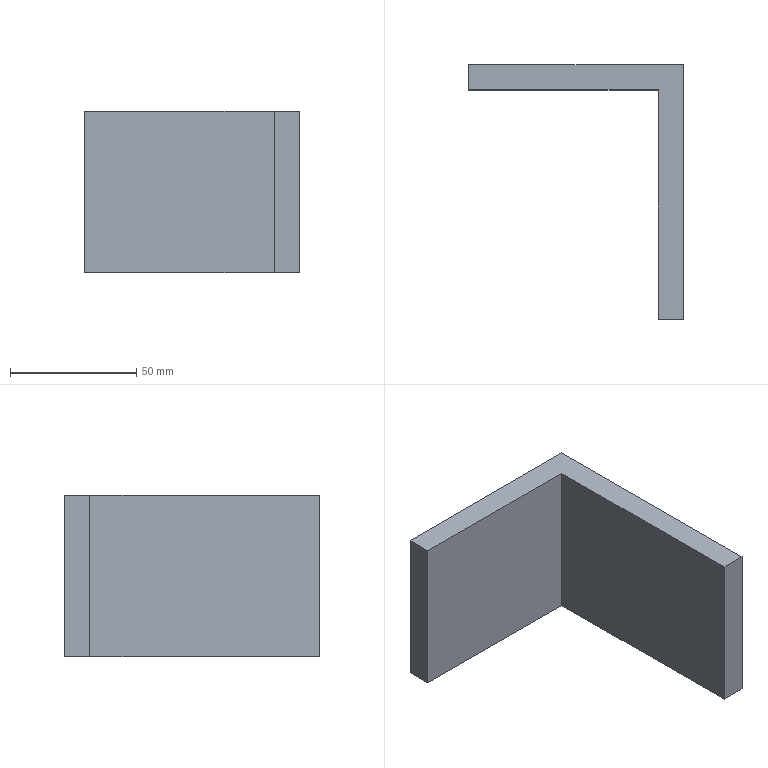Part | STEP file | Cylinder support plate | 1 solid | 8 faces | box 85 x 100.75 x 64 mm | volume 112480 mm3 | plane 8
STEP:
#1=CARTESIAN_POINT('',(0.,0.,0.));
#2=DIRECTION('',(0.,0.,1.));
#3=DIRECTION('',(1.,0.,0.));
#4=AXIS2_PLACEMENT_3D('',#1,#2,#3);
#5=CARTESIAN_POINT('',(85.,10.,64.));
#6=VERTEX_POINT('',#5);
#7=CARTESIAN_POINT('',(85.,10.,0.));
#8=VERTEX_POINT('',#7);
#9=CARTESIAN_POINT('',(85.,10.,64.));
#10=DIRECTION('',(0.,0.,-1.));
#11=VECTOR('',#10,1.);
#12=LINE('',#9,#11);
#13=CARTESIAN_POINT('',(85.,-90.75,64.));
#14=DIRECTION('',(-1.,0.,0.));
#15=DIRECTION('',(0.,0.,1.));
#16=AXIS2_PLACEMENT_3D('',#13,#14,#15);
#17=PLANE('',#16);
#18=CARTESIAN_POINT('',(0.,100.75));
#19=DIRECTION('',(-1.,0.));
#20=VECTOR('',#19,1.);
#21=LINE('',#18,#20);
#22=(GEOMETRIC_REPRESENTATION_CONTEXT(2)PARAMETRIC_REPRESENTATION_CONTEXT()REPRESENTATION_CONTEXT('',''));
#23=DEFINITIONAL_REPRESENTATION('',(#21),#22);
#24=PCURVE('',#17,#23);
#25=CARTESIAN_POINT('',(85.,10.,64.));
#26=DIRECTION('',(0.,-1.,0.));
#27=DIRECTION('',(1.,0.,0.));
#28=AXIS2_PLACEMENT_3D('',#25,#26,#27);
#29=PLANE('',#28);
#30=CARTESIAN_POINT('',(0.,0.));
#31=DIRECTION('',(0.,-1.));
#32=VECTOR('',#31,1.);
#33=LINE('',#30,#32);
#34=(GEOMETRIC_REPRESENTATION_CONTEXT(2)PARAMETRIC_REPRESENTATION_CONTEXT()REPRESENTATION_CONTEXT('',''));
#35=DEFINITIONAL_REPRESENTATION('',(#33),#34);
#36=PCURVE('',#29,#35);
#37=SURFACE_CURVE('',#12,(#24,#36),.PCURVE_S1.);
#38=EDGE_CURVE('',#6,#8,#37,.T.);
#39=ORIENTED_EDGE('',*,*,#38,.F.);
#40=CARTESIAN_POINT('',(85.,-90.75,64.));
#41=VERTEX_POINT('',#40);
#42=CARTESIAN_POINT('',(85.,-90.75,64.));
#43=DIRECTION('',(0.,1.,0.));
#44=VECTOR('',#43,1.);
#45=LINE('',#42,#44);
#46=CARTESIAN_POINT('',(0.,0.));
#47=DIRECTION('',(0.,1.));
#48=VECTOR('',#47,1.);
#49=LINE('',#46,#48);
#50=(GEOMETRIC_REPRESENTATION_CONTEXT(2)PARAMETRIC_REPRESENTATION_CONTEXT()REPRESENTATION_CONTEXT('',''));
#51=DEFINITIONAL_REPRESENTATION('',(#49),#50);
#52=PCURVE('',#17,#51);
#53=CARTESIAN_POINT('',(0.,0.,64.));
#54=DIRECTION('',(0.,0.,1.));
#55=DIRECTION('',(1.,0.,0.));
#56=AXIS2_PLACEMENT_3D('',#53,#54,#55);
#57=PLANE('',#56);
#58=CARTESIAN_POINT('',(85.,-90.75));
#59=DIRECTION('',(0.,1.));
#60=VECTOR('',#59,1.);
#61=LINE('',#58,#60);
#62=(GEOMETRIC_REPRESENTATION_CONTEXT(2)PARAMETRIC_REPRESENTATION_CONTEXT()REPRESENTATION_CONTEXT('',''));
#63=DEFINITIONAL_REPRESENTATION('',(#61),#62);
#64=PCURVE('',#57,#63);
#65=SURFACE_CURVE('',#45,(#52,#64),.PCURVE_S1.);
#66=EDGE_CURVE('',#41,#6,#65,.T.);
#67=ORIENTED_EDGE('',*,*,#66,.F.);
#68=CARTESIAN_POINT('',(85.,-90.75,0.));
#69=VERTEX_POINT('',#68);
#70=CARTESIAN_POINT('',(85.,-90.75,64.));
#71=DIRECTION('',(0.,0.,1.));
#72=VECTOR('',#71,1.);
#73=LINE('',#70,#72);
#74=CARTESIAN_POINT('',(0.,0.));
#75=DIRECTION('',(1.,0.));
#76=VECTOR('',#75,1.);
#77=LINE('',#74,#76);
#78=(GEOMETRIC_REPRESENTATION_CONTEXT(2)PARAMETRIC_REPRESENTATION_CONTEXT()REPRESENTATION_CONTEXT('',''));
#79=DEFINITIONAL_REPRESENTATION('',(#77),#78);
#80=PCURVE('',#17,#79);
#81=CARTESIAN_POINT('',(75.,-90.75,64.));
#82=DIRECTION('',(0.,1.,0.));
#83=DIRECTION('',(0.,0.,1.));
#84=AXIS2_PLACEMENT_3D('',#81,#82,#83);
#85=PLANE('',#84);
#86=CARTESIAN_POINT('',(0.,10.));
#87=DIRECTION('',(1.,0.));
#88=VECTOR('',#87,1.);
#89=LINE('',#86,#88);
#90=(GEOMETRIC_REPRESENTATION_CONTEXT(2)PARAMETRIC_REPRESENTATION_CONTEXT()REPRESENTATION_CONTEXT('',''));
#91=DEFINITIONAL_REPRESENTATION('',(#89),#90);
#92=PCURVE('',#85,#91);
#93=SURFACE_CURVE('',#73,(#80,#92),.PCURVE_S1.);
#94=EDGE_CURVE('',#69,#41,#93,.T.);
#95=ORIENTED_EDGE('',*,*,#94,.F.);
#96=CARTESIAN_POINT('',(85.,-90.75,0.));
#97=DIRECTION('',(0.,-1.,0.));
#98=VECTOR('',#97,1.);
#99=LINE('',#96,#98);
#100=CARTESIAN_POINT('',(-64.,0.));
#101=DIRECTION('',(0.,-1.));
#102=VECTOR('',#101,1.);
#103=LINE('',#100,#102);
#104=(GEOMETRIC_REPRESENTATION_CONTEXT(2)PARAMETRIC_REPRESENTATION_CONTEXT()REPRESENTATION_CONTEXT('',''));
#105=DEFINITIONAL_REPRESENTATION('',(#103),#104);
#106=PCURVE('',#17,#105);
#107=CARTESIAN_POINT('',(0.,0.,0.));
#108=DIRECTION('',(0.,0.,1.));
#109=DIRECTION('',(1.,0.,0.));
#110=AXIS2_PLACEMENT_3D('',#107,#108,#109);
#111=PLANE('',#110);
#112=CARTESIAN_POINT('',(85.,-90.75));
#113=DIRECTION('',(0.,-1.));
#114=VECTOR('',#113,1.);
#115=LINE('',#112,#114);
#116=(GEOMETRIC_REPRESENTATION_CONTEXT(2)PARAMETRIC_REPRESENTATION_CONTEXT()REPRESENTATION_CONTEXT('',''));
#117=DEFINITIONAL_REPRESENTATION('',(#115),#116);
#118=PCURVE('',#111,#117);
#119=SURFACE_CURVE('',#99,(#106,#118),.PCURVE_S1.);
#120=EDGE_CURVE('',#8,#69,#119,.T.);
#121=ORIENTED_EDGE('',*,*,#120,.F.);
#122=EDGE_LOOP('',(#39,#67,#95,#121));
#123=FACE_BOUND('',#122,.T.);
#124=ADVANCED_FACE('',(#123),#17,.F.);
#125=CARTESIAN_POINT('',(0.,10.,0.));
#126=VERTEX_POINT('',#125);
#127=CARTESIAN_POINT('',(0.,10.,0.));
#128=DIRECTION('',(-1.,0.,0.));
#129=VECTOR('',#128,1.);
#130=LINE('',#127,#129);
#131=CARTESIAN_POINT('',(0.,10.));
#132=DIRECTION('',(-1.,0.));
#133=VECTOR('',#132,1.);
#134=LINE('',#131,#133);
#135=(GEOMETRIC_REPRESENTATION_CONTEXT(2)PARAMETRIC_REPRESENTATION_CONTEXT()REPRESENTATION_CONTEXT('',''));
#136=DEFINITIONAL_REPRESENTATION('',(#134),#135);
#137=PCURVE('',#111,#136);
#138=CARTESIAN_POINT('',(-85.,-64.));
#139=DIRECTION('',(-1.,0.));
#140=VECTOR('',#139,1.);
#141=LINE('',#138,#140);
#142=(GEOMETRIC_REPRESENTATION_CONTEXT(2)PARAMETRIC_REPRESENTATION_CONTEXT()REPRESENTATION_CONTEXT('',''));
#143=DEFINITIONAL_REPRESENTATION('',(#141),#142);
#144=PCURVE('',#29,#143);
#145=SURFACE_CURVE('',#130,(#137,#144),.PCURVE_S1.);
#146=EDGE_CURVE('',#8,#126,#145,.T.);
#147=ORIENTED_EDGE('',*,*,#146,.F.);
#148=ORIENTED_EDGE('',*,*,#120,.T.);
#149=CARTESIAN_POINT('',(75.,-90.75,0.));
#150=VERTEX_POINT('',#149);
#151=CARTESIAN_POINT('',(0.,-90.75,0.));
#152=DIRECTION('',(1.,0.,0.));
#153=VECTOR('',#152,1.);
#154=LINE('',#151,#153);
#155=CARTESIAN_POINT('',(0.,-90.75));
#156=DIRECTION('',(1.,0.));
#157=VECTOR('',#156,1.);
#158=LINE('',#155,#157);
#159=(GEOMETRIC_REPRESENTATION_CONTEXT(2)PARAMETRIC_REPRESENTATION_CONTEXT()REPRESENTATION_CONTEXT('',''));
#160=DEFINITIONAL_REPRESENTATION('',(#158),#159);
#161=PCURVE('',#111,#160);
#162=CARTESIAN_POINT('',(-64.,-75.));
#163=DIRECTION('',(0.,1.));
#164=VECTOR('',#163,1.);
#165=LINE('',#162,#164);
#166=(GEOMETRIC_REPRESENTATION_CONTEXT(2)PARAMETRIC_REPRESENTATION_CONTEXT()REPRESENTATION_CONTEXT('',''));
#167=DEFINITIONAL_REPRESENTATION('',(#165),#166);
#168=PCURVE('',#85,#167);
#169=SURFACE_CURVE('',#154,(#161,#168),.PCURVE_S1.);
#170=EDGE_CURVE('',#150,#69,#169,.T.);
#171=ORIENTED_EDGE('',*,*,#170,.F.);
#172=CARTESIAN_POINT('',(75.,0.,0.));
#173=VERTEX_POINT('',#172);
#174=CARTESIAN_POINT('',(75.,0.,0.));
#175=DIRECTION('',(0.,-1.,0.));
#176=VECTOR('',#175,1.);
#177=LINE('',#174,#176);
#178=CARTESIAN_POINT('',(75.,0.));
#179=DIRECTION('',(0.,-1.));
#180=VECTOR('',#179,1.);
#181=LINE('',#178,#180);
#182=(GEOMETRIC_REPRESENTATION_CONTEXT(2)PARAMETRIC_REPRESENTATION_CONTEXT()REPRESENTATION_CONTEXT('',''));
#183=DEFINITIONAL_REPRESENTATION('',(#181),#182);
#184=PCURVE('',#111,#183);
#185=CARTESIAN_POINT('',(75.,0.,64.));
#186=DIRECTION('',(1.,0.,0.));
#187=DIRECTION('',(0.,1.,0.));
#188=AXIS2_PLACEMENT_3D('',#185,#186,#187);
#189=PLANE('',#188);
#190=CARTESIAN_POINT('',(0.,-64.));
#191=DIRECTION('',(-1.,0.));
#192=VECTOR('',#191,1.);
#193=LINE('',#190,#192);
#194=(GEOMETRIC_REPRESENTATION_CONTEXT(2)PARAMETRIC_REPRESENTATION_CONTEXT()REPRESENTATION_CONTEXT('',''));
#195=DEFINITIONAL_REPRESENTATION('',(#193),#194);
#196=PCURVE('',#189,#195);
#197=SURFACE_CURVE('',#177,(#184,#196),.PCURVE_S1.);
#198=EDGE_CURVE('',#173,#150,#197,.T.);
#199=ORIENTED_EDGE('',*,*,#198,.F.);
#200=CARTESIAN_POINT('',(0.,0.,0.));
#201=VERTEX_POINT('',#200);
#202=CARTESIAN_POINT('',(0.,0.,0.));
#203=DIRECTION('',(1.,0.,0.));
#204=VECTOR('',#203,1.);
#205=LINE('',#202,#204);
#206=CARTESIAN_POINT('',(0.,0.));
#207=DIRECTION('',(1.,0.));
#208=VECTOR('',#207,1.);
#209=LINE('',#206,#208);
#210=(GEOMETRIC_REPRESENTATION_CONTEXT(2)PARAMETRIC_REPRESENTATION_CONTEXT()REPRESENTATION_CONTEXT('',''));
#211=DEFINITIONAL_REPRESENTATION('',(#209),#210);
#212=PCURVE('',#111,#211);
#213=CARTESIAN_POINT('',(0.,0.,64.));
#214=DIRECTION('',(0.,1.,0.));
#215=DIRECTION('',(0.,0.,1.));
#216=AXIS2_PLACEMENT_3D('',#213,#214,#215);
#217=PLANE('',#216);
#218=CARTESIAN_POINT('',(-64.,0.));
#219=DIRECTION('',(0.,1.));
#220=VECTOR('',#219,1.);
#221=LINE('',#218,#220);
#222=(GEOMETRIC_REPRESENTATION_CONTEXT(2)PARAMETRIC_REPRESENTATION_CONTEXT()REPRESENTATION_CONTEXT('',''));
#223=DEFINITIONAL_REPRESENTATION('',(#221),#222);
#224=PCURVE('',#217,#223);
#225=SURFACE_CURVE('',#205,(#212,#224),.PCURVE_S1.);
#226=EDGE_CURVE('',#201,#173,#225,.T.);
#227=ORIENTED_EDGE('',*,*,#226,.F.);
#228=CARTESIAN_POINT('',(0.,0.,0.));
#229=DIRECTION('',(0.,-1.,0.));
#230=VECTOR('',#229,1.);
#231=LINE('',#228,#230);
#232=CARTESIAN_POINT('',(0.,0.));
#233=DIRECTION('',(0.,-1.));
#234=VECTOR('',#233,1.);
#235=LINE('',#232,#234);
#236=(GEOMETRIC_REPRESENTATION_CONTEXT(2)PARAMETRIC_REPRESENTATION_CONTEXT()REPRESENTATION_CONTEXT('',''));
#237=DEFINITIONAL_REPRESENTATION('',(#235),#236);
#238=PCURVE('',#111,#237);
#239=CARTESIAN_POINT('',(0.,10.,64.));
#240=DIRECTION('',(1.,0.,0.));
#241=DIRECTION('',(0.,1.,0.));
#242=AXIS2_PLACEMENT_3D('',#239,#240,#241);
#243=PLANE('',#242);
#244=CARTESIAN_POINT('',(-10.,-64.));
#245=DIRECTION('',(-1.,0.));
#246=VECTOR('',#245,1.);
#247=LINE('',#244,#246);
#248=(GEOMETRIC_REPRESENTATION_CONTEXT(2)PARAMETRIC_REPRESENTATION_CONTEXT()REPRESENTATION_CONTEXT('',''));
#249=DEFINITIONAL_REPRESENTATION('',(#247),#248);
#250=PCURVE('',#243,#249);
#251=SURFACE_CURVE('',#231,(#238,#250),.PCURVE_S1.);
#252=EDGE_CURVE('',#126,#201,#251,.T.);
#253=ORIENTED_EDGE('',*,*,#252,.F.);
#254=EDGE_LOOP('',(#147,#148,#171,#199,#227,#253));
#255=FACE_BOUND('',#254,.T.);
#256=ADVANCED_FACE('',(#255),#111,.F.);
#257=CARTESIAN_POINT('',(0.,10.,64.));
#258=VERTEX_POINT('',#257);
#259=CARTESIAN_POINT('',(0.,10.,64.));
#260=DIRECTION('',(0.,0.,-1.));
#261=VECTOR('',#260,1.);
#262=LINE('',#259,#261);
#263=CARTESIAN_POINT('',(-85.,0.));
#264=DIRECTION('',(0.,-1.));
#265=VECTOR('',#264,1.);
#266=LINE('',#263,#265);
#267=(GEOMETRIC_REPRESENTATION_CONTEXT(2)PARAMETRIC_REPRESENTATION_CONTEXT()REPRESENTATION_CONTEXT('',''));
#268=DEFINITIONAL_REPRESENTATION('',(#266),#267);
#269=PCURVE('',#29,#268);
#270=CARTESIAN_POINT('',(0.,0.));
#271=DIRECTION('',(0.,-1.));
#272=VECTOR('',#271,1.);
#273=LINE('',#270,#272);
#274=(GEOMETRIC_REPRESENTATION_CONTEXT(2)PARAMETRIC_REPRESENTATION_CONTEXT()REPRESENTATION_CONTEXT('',''));
#275=DEFINITIONAL_REPRESENTATION('',(#273),#274);
#276=PCURVE('',#243,#275);
#277=SURFACE_CURVE('',#262,(#269,#276),.PCURVE_S1.);
#278=EDGE_CURVE('',#258,#126,#277,.T.);
#279=ORIENTED_EDGE('',*,*,#278,.F.);
#280=CARTESIAN_POINT('',(85.,10.,64.));
#281=DIRECTION('',(-1.,0.,0.));
#282=VECTOR('',#281,1.);
#283=LINE('',#280,#282);
#284=CARTESIAN_POINT('',(0.,0.));
#285=DIRECTION('',(-1.,0.));
#286=VECTOR('',#285,1.);
#287=LINE('',#284,#286);
#288=(GEOMETRIC_REPRESENTATION_CONTEXT(2)PARAMETRIC_REPRESENTATION_CONTEXT()REPRESENTATION_CONTEXT('',''));
#289=DEFINITIONAL_REPRESENTATION('',(#287),#288);
#290=PCURVE('',#29,#289);
#291=CARTESIAN_POINT('',(85.,10.));
#292=DIRECTION('',(-1.,0.));
#293=VECTOR('',#292,1.);
#294=LINE('',#291,#293);
#295=(GEOMETRIC_REPRESENTATION_CONTEXT(2)PARAMETRIC_REPRESENTATION_CONTEXT()REPRESENTATION_CONTEXT('',''));
#296=DEFINITIONAL_REPRESENTATION('',(#294),#295);
#297=PCURVE('',#57,#296);
#298=SURFACE_CURVE('',#283,(#290,#297),.PCURVE_S1.);
#299=EDGE_CURVE('',#6,#258,#298,.T.);
#300=ORIENTED_EDGE('',*,*,#299,.F.);
#301=ORIENTED_EDGE('',*,*,#38,.T.);
#302=ORIENTED_EDGE('',*,*,#146,.T.);
#303=EDGE_LOOP('',(#279,#300,#301,#302));
#304=FACE_BOUND('',#303,.T.);
#305=ADVANCED_FACE('',(#304),#29,.F.);
#306=ORIENTED_EDGE('',*,*,#66,.T.);
#307=ORIENTED_EDGE('',*,*,#299,.T.);
#308=CARTESIAN_POINT('',(0.,0.,64.));
#309=VERTEX_POINT('',#308);
#310=CARTESIAN_POINT('',(0.,0.,64.));
#311=DIRECTION('',(0.,-1.,0.));
#312=VECTOR('',#311,1.);
#313=LINE('',#310,#312);
#314=CARTESIAN_POINT('',(0.,0.));
#315=DIRECTION('',(0.,-1.));
#316=VECTOR('',#315,1.);
#317=LINE('',#314,#316);
#318=(GEOMETRIC_REPRESENTATION_CONTEXT(2)PARAMETRIC_REPRESENTATION_CONTEXT()REPRESENTATION_CONTEXT('',''));
#319=DEFINITIONAL_REPRESENTATION('',(#317),#318);
#320=PCURVE('',#57,#319);
#321=CARTESIAN_POINT('',(-10.,0.));
#322=DIRECTION('',(-1.,0.));
#323=VECTOR('',#322,1.);
#324=LINE('',#321,#323);
#325=(GEOMETRIC_REPRESENTATION_CONTEXT(2)PARAMETRIC_REPRESENTATION_CONTEXT()REPRESENTATION_CONTEXT('',''));
#326=DEFINITIONAL_REPRESENTATION('',(#324),#325);
#327=PCURVE('',#243,#326);
#328=SURFACE_CURVE('',#313,(#320,#327),.PCURVE_S1.);
#329=EDGE_CURVE('',#258,#309,#328,.T.);
#330=ORIENTED_EDGE('',*,*,#329,.T.);
#331=CARTESIAN_POINT('',(75.,0.,64.));
#332=VERTEX_POINT('',#331);
#333=CARTESIAN_POINT('',(0.,0.,64.));
#334=DIRECTION('',(1.,0.,0.));
#335=VECTOR('',#334,1.);
#336=LINE('',#333,#335);
#337=CARTESIAN_POINT('',(0.,0.));
#338=DIRECTION('',(1.,0.));
#339=VECTOR('',#338,1.);
#340=LINE('',#337,#339);
#341=(GEOMETRIC_REPRESENTATION_CONTEXT(2)PARAMETRIC_REPRESENTATION_CONTEXT()REPRESENTATION_CONTEXT('',''));
#342=DEFINITIONAL_REPRESENTATION('',(#340),#341);
#343=PCURVE('',#57,#342);
#344=CARTESIAN_POINT('',(0.,0.));
#345=DIRECTION('',(0.,1.));
#346=VECTOR('',#345,1.);
#347=LINE('',#344,#346);
#348=(GEOMETRIC_REPRESENTATION_CONTEXT(2)PARAMETRIC_REPRESENTATION_CONTEXT()REPRESENTATION_CONTEXT('',''));
#349=DEFINITIONAL_REPRESENTATION('',(#347),#348);
#350=PCURVE('',#217,#349);
#351=SURFACE_CURVE('',#336,(#343,#350),.PCURVE_S1.);
#352=EDGE_CURVE('',#309,#332,#351,.T.);
#353=ORIENTED_EDGE('',*,*,#352,.T.);
#354=CARTESIAN_POINT('',(75.,-90.75,64.));
#355=VERTEX_POINT('',#354);
#356=CARTESIAN_POINT('',(75.,0.,64.));
#357=DIRECTION('',(0.,-1.,0.));
#358=VECTOR('',#357,1.);
#359=LINE('',#356,#358);
#360=CARTESIAN_POINT('',(75.,0.));
#361=DIRECTION('',(0.,-1.));
#362=VECTOR('',#361,1.);
#363=LINE('',#360,#362);
#364=(GEOMETRIC_REPRESENTATION_CONTEXT(2)PARAMETRIC_REPRESENTATION_CONTEXT()REPRESENTATION_CONTEXT('',''));
#365=DEFINITIONAL_REPRESENTATION('',(#363),#364);
#366=PCURVE('',#57,#365);
#367=CARTESIAN_POINT('',(0.,0.));
#368=DIRECTION('',(-1.,0.));
#369=VECTOR('',#368,1.);
#370=LINE('',#367,#369);
#371=(GEOMETRIC_REPRESENTATION_CONTEXT(2)PARAMETRIC_REPRESENTATION_CONTEXT()REPRESENTATION_CONTEXT('',''));
#372=DEFINITIONAL_REPRESENTATION('',(#370),#371);
#373=PCURVE('',#189,#372);
#374=SURFACE_CURVE('',#359,(#366,#373),.PCURVE_S1.);
#375=EDGE_CURVE('',#332,#355,#374,.T.);
#376=ORIENTED_EDGE('',*,*,#375,.T.);
#377=CARTESIAN_POINT('',(0.,-90.75,64.));
#378=DIRECTION('',(1.,0.,0.));
#379=VECTOR('',#378,1.);
#380=LINE('',#377,#379);
#381=CARTESIAN_POINT('',(0.,-90.75));
#382=DIRECTION('',(1.,0.));
#383=VECTOR('',#382,1.);
#384=LINE('',#381,#383);
#385=(GEOMETRIC_REPRESENTATION_CONTEXT(2)PARAMETRIC_REPRESENTATION_CONTEXT()REPRESENTATION_CONTEXT('',''));
#386=DEFINITIONAL_REPRESENTATION('',(#384),#385);
#387=PCURVE('',#57,#386);
#388=CARTESIAN_POINT('',(0.,-75.));
#389=DIRECTION('',(0.,1.));
#390=VECTOR('',#389,1.);
#391=LINE('',#388,#390);
#392=(GEOMETRIC_REPRESENTATION_CONTEXT(2)PARAMETRIC_REPRESENTATION_CONTEXT()REPRESENTATION_CONTEXT('',''));
#393=DEFINITIONAL_REPRESENTATION('',(#391),#392);
#394=PCURVE('',#85,#393);
#395=SURFACE_CURVE('',#380,(#387,#394),.PCURVE_S1.);
#396=EDGE_CURVE('',#355,#41,#395,.T.);
#397=ORIENTED_EDGE('',*,*,#396,.T.);
#398=EDGE_LOOP('',(#306,#307,#330,#353,#376,#397));
#399=FACE_BOUND('',#398,.T.);
#400=ADVANCED_FACE('',(#399),#57,.T.);
#401=ORIENTED_EDGE('',*,*,#94,.T.);
#402=ORIENTED_EDGE('',*,*,#396,.F.);
#403=CARTESIAN_POINT('',(75.,-90.75,64.));
#404=DIRECTION('',(0.,0.,1.));
#405=VECTOR('',#404,1.);
#406=LINE('',#403,#405);
#407=CARTESIAN_POINT('',(0.,0.));
#408=DIRECTION('',(1.,0.));
#409=VECTOR('',#408,1.);
#410=LINE('',#407,#409);
#411=(GEOMETRIC_REPRESENTATION_CONTEXT(2)PARAMETRIC_REPRESENTATION_CONTEXT()REPRESENTATION_CONTEXT('',''));
#412=DEFINITIONAL_REPRESENTATION('',(#410),#411);
#413=PCURVE('',#85,#412);
#414=CARTESIAN_POINT('',(-90.75,0.));
#415=DIRECTION('',(0.,1.));
#416=VECTOR('',#415,1.);
#417=LINE('',#414,#416);
#418=(GEOMETRIC_REPRESENTATION_CONTEXT(2)PARAMETRIC_REPRESENTATION_CONTEXT()REPRESENTATION_CONTEXT('',''));
#419=DEFINITIONAL_REPRESENTATION('',(#417),#418);
#420=PCURVE('',#189,#419);
#421=SURFACE_CURVE('',#406,(#413,#420),.PCURVE_S1.);
#422=EDGE_CURVE('',#150,#355,#421,.T.);
#423=ORIENTED_EDGE('',*,*,#422,.F.);
#424=ORIENTED_EDGE('',*,*,#170,.T.);
#425=EDGE_LOOP('',(#401,#402,#423,#424));
#426=FACE_BOUND('',#425,.T.);
#427=ADVANCED_FACE('',(#426),#85,.F.);
#428=CARTESIAN_POINT('',(0.,0.,64.));
#429=DIRECTION('',(0.,0.,-1.));
#430=VECTOR('',#429,1.);
#431=LINE('',#428,#430);
#432=CARTESIAN_POINT('',(-10.,0.));
#433=DIRECTION('',(0.,-1.));
#434=VECTOR('',#433,1.);
#435=LINE('',#432,#434);
#436=(GEOMETRIC_REPRESENTATION_CONTEXT(2)PARAMETRIC_REPRESENTATION_CONTEXT()REPRESENTATION_CONTEXT('',''));
#437=DEFINITIONAL_REPRESENTATION('',(#435),#436);
#438=PCURVE('',#243,#437);
#439=CARTESIAN_POINT('',(0.,0.));
#440=DIRECTION('',(-1.,0.));
#441=VECTOR('',#440,1.);
#442=LINE('',#439,#441);
#443=(GEOMETRIC_REPRESENTATION_CONTEXT(2)PARAMETRIC_REPRESENTATION_CONTEXT()REPRESENTATION_CONTEXT('',''));
#444=DEFINITIONAL_REPRESENTATION('',(#442),#443);
#445=PCURVE('',#217,#444);
#446=SURFACE_CURVE('',#431,(#438,#445),.PCURVE_S1.);
#447=EDGE_CURVE('',#309,#201,#446,.T.);
#448=ORIENTED_EDGE('',*,*,#447,.F.);
#449=ORIENTED_EDGE('',*,*,#329,.F.);
#450=ORIENTED_EDGE('',*,*,#278,.T.);
#451=ORIENTED_EDGE('',*,*,#252,.T.);
#452=EDGE_LOOP('',(#448,#449,#450,#451));
#453=FACE_BOUND('',#452,.T.);
#454=ADVANCED_FACE('',(#453),#243,.F.);
#455=ORIENTED_EDGE('',*,*,#422,.T.);
#456=ORIENTED_EDGE('',*,*,#375,.F.);
#457=CARTESIAN_POINT('',(75.,0.,64.));
#458=DIRECTION('',(0.,0.,1.));
#459=VECTOR('',#458,1.);
#460=LINE('',#457,#459);
#461=CARTESIAN_POINT('',(0.,0.));
#462=DIRECTION('',(0.,1.));
#463=VECTOR('',#462,1.);
#464=LINE('',#461,#463);
#465=(GEOMETRIC_REPRESENTATION_CONTEXT(2)PARAMETRIC_REPRESENTATION_CONTEXT()REPRESENTATION_CONTEXT('',''));
#466=DEFINITIONAL_REPRESENTATION('',(#464),#465);
#467=PCURVE('',#189,#466);
#468=CARTESIAN_POINT('',(0.,75.));
#469=DIRECTION('',(1.,0.));
#470=VECTOR('',#469,1.);
#471=LINE('',#468,#470);
#472=(GEOMETRIC_REPRESENTATION_CONTEXT(2)PARAMETRIC_REPRESENTATION_CONTEXT()REPRESENTATION_CONTEXT('',''));
#473=DEFINITIONAL_REPRESENTATION('',(#471),#472);
#474=PCURVE('',#217,#473);
#475=SURFACE_CURVE('',#460,(#467,#474),.PCURVE_S1.);
#476=EDGE_CURVE('',#173,#332,#475,.T.);
#477=ORIENTED_EDGE('',*,*,#476,.F.);
#478=ORIENTED_EDGE('',*,*,#198,.T.);
#479=EDGE_LOOP('',(#455,#456,#477,#478));
#480=FACE_BOUND('',#479,.T.);
#481=ADVANCED_FACE('',(#480),#189,.F.);
#482=ORIENTED_EDGE('',*,*,#476,.T.);
#483=ORIENTED_EDGE('',*,*,#352,.F.);
#484=ORIENTED_EDGE('',*,*,#447,.T.);
#485=ORIENTED_EDGE('',*,*,#226,.T.);
#486=EDGE_LOOP('',(#482,#483,#484,#485));
#487=FACE_BOUND('',#486,.T.);
#488=ADVANCED_FACE('',(#487),#217,.F.);
#489=CLOSED_SHELL('',(#124,#256,#305,#400,#427,#454,#481,#488));
#490=MANIFOLD_SOLID_BREP('',#489);
#491=(LENGTH_UNIT()NAMED_UNIT(*)SI_UNIT(.MILLI.,.METRE.));
#492=UNCERTAINTY_MEASURE_WITH_UNIT(LENGTH_MEASURE(0.0000001),#491,'','');
#493=(NAMED_UNIT(*)PLANE_ANGLE_UNIT()SI_UNIT($,.RADIAN.));
#494=(NAMED_UNIT(*)SI_UNIT($,.STERADIAN.)SOLID_ANGLE_UNIT());
#495=(GEOMETRIC_REPRESENTATION_CONTEXT(3)GLOBAL_UNCERTAINTY_ASSIGNED_CONTEXT((#492))GLOBAL_UNIT_ASSIGNED_CONTEXT((#491,#493,#494))REPRESENTATION_CONTEXT('',''));
#496=ADVANCED_BREP_SHAPE_REPRESENTATION('',(#4,#490),#495);